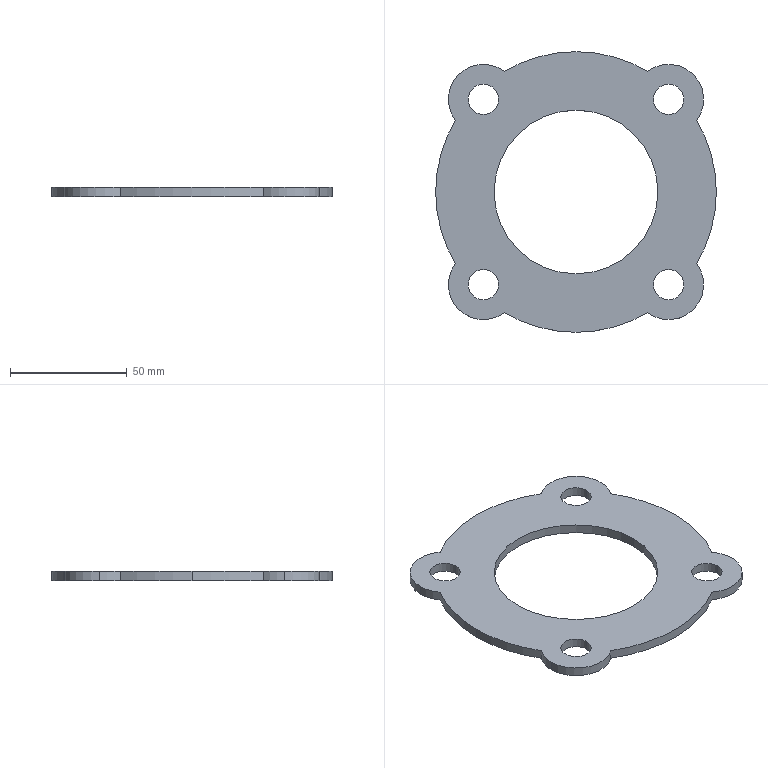Part | SolidWorks | features Extrusion 1 | 1 solid | 23 faces | box 120 x 120 x 4 mm | volume 31763 mm3 | cylinder 21 | plane 2 | commonest cylinder face diameters 13 x8 30 x6 120 x5 70 x2
STEP:
#1=CARTESIAN_POINT('',(-35.,0.,2.));
#2=VERTEX_POINT('',#1);
#3=CARTESIAN_POINT('',(35.,0.,2.));
#4=VERTEX_POINT('',#3);
#5=CARTESIAN_POINT('',(0.,0.,2.));
#6=DIRECTION('',(0.,0.,1.));
#7=DIRECTION('',(1.,0.,0.));
#8=AXIS2_PLACEMENT_3D('',#5,#6,#7);
#9=CIRCLE('',#8,35.);
#10=EDGE_CURVE('',#2,#4,#9,.T.);
#11=ORIENTED_EDGE('',*,*,#10,.T.);
#12=CARTESIAN_POINT('',(35.,0.,-2.));
#13=VERTEX_POINT('',#12);
#14=CARTESIAN_POINT('',(35.,0.,2.));
#15=DIRECTION('',(0.,0.,-1.));
#16=VECTOR('',#15,1000.);
#17=LINE('',#14,#16);
#18=EDGE_CURVE('',#4,#13,#17,.T.);
#19=ORIENTED_EDGE('',*,*,#18,.T.);
#20=CARTESIAN_POINT('',(-35.,0.,-2.));
#21=VERTEX_POINT('',#20);
#22=CARTESIAN_POINT('',(0.,0.,-2.));
#23=DIRECTION('',(0.,0.,1.));
#24=DIRECTION('',(1.,0.,0.));
#25=AXIS2_PLACEMENT_3D('',#22,#23,#24);
#26=CIRCLE('',#25,35.);
#27=EDGE_CURVE('',#21,#13,#26,.T.);
#28=ORIENTED_EDGE('',*,*,#27,.F.);
#29=CARTESIAN_POINT('',(-35.,0.,2.));
#30=DIRECTION('',(0.,0.,-1.));
#31=VECTOR('',#30,1000.);
#32=LINE('',#29,#31);
#33=EDGE_CURVE('',#2,#21,#32,.T.);
#34=ORIENTED_EDGE('',*,*,#33,.F.);
#35=EDGE_LOOP('',(#11,#19,#28,#34));
#36=FACE_OUTER_BOUND('',#35,.T.);
#37=CARTESIAN_POINT('',(0.,0.,2.));
#38=DIRECTION('',(0.,0.,-1.));
#39=DIRECTION('',(-1.,0.,0.));
#40=AXIS2_PLACEMENT_3D('',#37,#38,#39);
#41=CYLINDRICAL_SURFACE('',#40,35.);
#42=ADVANCED_FACE('',(#36),#41,.F.);
#43=CARTESIAN_POINT('',(33.098,39.598,2.));
#44=VERTEX_POINT('',#43);
#45=CARTESIAN_POINT('',(46.098,39.598,2.));
#46=VERTEX_POINT('',#45);
#47=CARTESIAN_POINT('',(39.598,39.598,2.));
#48=DIRECTION('',(0.,0.,1.));
#49=DIRECTION('',(1.,0.,0.));
#50=AXIS2_PLACEMENT_3D('',#47,#48,#49);
#51=CIRCLE('',#50,6.5);
#52=EDGE_CURVE('',#44,#46,#51,.T.);
#53=ORIENTED_EDGE('',*,*,#52,.T.);
#54=CARTESIAN_POINT('',(46.098,39.598,-2.));
#55=VERTEX_POINT('',#54);
#56=CARTESIAN_POINT('',(46.098,39.598,2.));
#57=DIRECTION('',(0.,0.,-1.));
#58=VECTOR('',#57,1000.);
#59=LINE('',#56,#58);
#60=EDGE_CURVE('',#46,#55,#59,.T.);
#61=ORIENTED_EDGE('',*,*,#60,.T.);
#62=CARTESIAN_POINT('',(33.098,39.598,-2.));
#63=VERTEX_POINT('',#62);
#64=CARTESIAN_POINT('',(39.598,39.598,-2.));
#65=DIRECTION('',(0.,0.,1.));
#66=DIRECTION('',(1.,0.,0.));
#67=AXIS2_PLACEMENT_3D('',#64,#65,#66);
#68=CIRCLE('',#67,6.5);
#69=EDGE_CURVE('',#63,#55,#68,.T.);
#70=ORIENTED_EDGE('',*,*,#69,.F.);
#71=CARTESIAN_POINT('',(33.098,39.598,2.));
#72=DIRECTION('',(0.,0.,-1.));
#73=VECTOR('',#72,1000.);
#74=LINE('',#71,#73);
#75=EDGE_CURVE('',#44,#63,#74,.T.);
#76=ORIENTED_EDGE('',*,*,#75,.F.);
#77=EDGE_LOOP('',(#53,#61,#70,#76));
#78=FACE_OUTER_BOUND('',#77,.T.);
#79=CARTESIAN_POINT('',(39.598,39.598,2.));
#80=DIRECTION('',(0.,0.,-1.));
#81=DIRECTION('',(-1.,0.,0.));
#82=AXIS2_PLACEMENT_3D('',#79,#80,#81);
#83=CYLINDRICAL_SURFACE('',#82,6.5);
#84=ADVANCED_FACE('',(#78),#83,.F.);
#85=CARTESIAN_POINT('',(33.098,-39.598,2.));
#86=VERTEX_POINT('',#85);
#87=CARTESIAN_POINT('',(46.098,-39.598,2.));
#88=VERTEX_POINT('',#87);
#89=CARTESIAN_POINT('',(39.598,-39.598,2.));
#90=DIRECTION('',(0.,0.,1.));
#91=DIRECTION('',(1.,0.,0.));
#92=AXIS2_PLACEMENT_3D('',#89,#90,#91);
#93=CIRCLE('',#92,6.5);
#94=EDGE_CURVE('',#86,#88,#93,.T.);
#95=ORIENTED_EDGE('',*,*,#94,.T.);
#96=CARTESIAN_POINT('',(46.098,-39.598,-2.));
#97=VERTEX_POINT('',#96);
#98=CARTESIAN_POINT('',(46.098,-39.598,2.));
#99=DIRECTION('',(0.,0.,-1.));
#100=VECTOR('',#99,1000.);
#101=LINE('',#98,#100);
#102=EDGE_CURVE('',#88,#97,#101,.T.);
#103=ORIENTED_EDGE('',*,*,#102,.T.);
#104=CARTESIAN_POINT('',(33.098,-39.598,-2.));
#105=VERTEX_POINT('',#104);
#106=CARTESIAN_POINT('',(39.598,-39.598,-2.));
#107=DIRECTION('',(0.,0.,1.));
#108=DIRECTION('',(1.,0.,0.));
#109=AXIS2_PLACEMENT_3D('',#106,#107,#108);
#110=CIRCLE('',#109,6.5);
#111=EDGE_CURVE('',#105,#97,#110,.T.);
#112=ORIENTED_EDGE('',*,*,#111,.F.);
#113=CARTESIAN_POINT('',(33.098,-39.598,2.));
#114=DIRECTION('',(0.,0.,-1.));
#115=VECTOR('',#114,1000.);
#116=LINE('',#113,#115);
#117=EDGE_CURVE('',#86,#105,#116,.T.);
#118=ORIENTED_EDGE('',*,*,#117,.F.);
#119=EDGE_LOOP('',(#95,#103,#112,#118));
#120=FACE_OUTER_BOUND('',#119,.T.);
#121=CARTESIAN_POINT('',(39.598,-39.598,2.));
#122=DIRECTION('',(0.,0.,-1.));
#123=DIRECTION('',(-1.,0.,0.));
#124=AXIS2_PLACEMENT_3D('',#121,#122,#123);
#125=CYLINDRICAL_SURFACE('',#124,6.5);
#126=ADVANCED_FACE('',(#120),#125,.F.);
#127=CARTESIAN_POINT('',(-46.098,-39.598,2.));
#128=VERTEX_POINT('',#127);
#129=CARTESIAN_POINT('',(-33.098,-39.598,2.));
#130=VERTEX_POINT('',#129);
#131=CARTESIAN_POINT('',(-39.598,-39.598,2.));
#132=DIRECTION('',(0.,0.,1.));
#133=DIRECTION('',(1.,0.,0.));
#134=AXIS2_PLACEMENT_3D('',#131,#132,#133);
#135=CIRCLE('',#134,6.5);
#136=EDGE_CURVE('',#128,#130,#135,.T.);
#137=ORIENTED_EDGE('',*,*,#136,.T.);
#138=CARTESIAN_POINT('',(-33.098,-39.598,-2.));
#139=VERTEX_POINT('',#138);
#140=CARTESIAN_POINT('',(-33.098,-39.598,2.));
#141=DIRECTION('',(0.,0.,-1.));
#142=VECTOR('',#141,1000.);
#143=LINE('',#140,#142);
#144=EDGE_CURVE('',#130,#139,#143,.T.);
#145=ORIENTED_EDGE('',*,*,#144,.T.);
#146=CARTESIAN_POINT('',(-46.098,-39.598,-2.));
#147=VERTEX_POINT('',#146);
#148=CARTESIAN_POINT('',(-39.598,-39.598,-2.));
#149=DIRECTION('',(0.,0.,1.));
#150=DIRECTION('',(1.,0.,0.));
#151=AXIS2_PLACEMENT_3D('',#148,#149,#150);
#152=CIRCLE('',#151,6.5);
#153=EDGE_CURVE('',#147,#139,#152,.T.);
#154=ORIENTED_EDGE('',*,*,#153,.F.);
#155=CARTESIAN_POINT('',(-46.098,-39.598,2.));
#156=DIRECTION('',(0.,0.,-1.));
#157=VECTOR('',#156,1000.);
#158=LINE('',#155,#157);
#159=EDGE_CURVE('',#128,#147,#158,.T.);
#160=ORIENTED_EDGE('',*,*,#159,.F.);
#161=EDGE_LOOP('',(#137,#145,#154,#160));
#162=FACE_OUTER_BOUND('',#161,.T.);
#163=CARTESIAN_POINT('',(-39.598,-39.598,2.));
#164=DIRECTION('',(0.,0.,-1.));
#165=DIRECTION('',(-1.,0.,0.));
#166=AXIS2_PLACEMENT_3D('',#163,#164,#165);
#167=CYLINDRICAL_SURFACE('',#166,6.5);
#168=ADVANCED_FACE('',(#162),#167,.F.);
#169=CARTESIAN_POINT('',(-46.098,39.598,2.));
#170=VERTEX_POINT('',#169);
#171=CARTESIAN_POINT('',(-33.098,39.598,2.));
#172=VERTEX_POINT('',#171);
#173=CARTESIAN_POINT('',(-39.598,39.598,2.));
#174=DIRECTION('',(0.,0.,1.));
#175=DIRECTION('',(1.,0.,0.));
#176=AXIS2_PLACEMENT_3D('',#173,#174,#175);
#177=CIRCLE('',#176,6.5);
#178=EDGE_CURVE('',#170,#172,#177,.T.);
#179=ORIENTED_EDGE('',*,*,#178,.T.);
#180=CARTESIAN_POINT('',(-33.098,39.598,-2.));
#181=VERTEX_POINT('',#180);
#182=CARTESIAN_POINT('',(-33.098,39.598,2.));
#183=DIRECTION('',(0.,0.,-1.));
#184=VECTOR('',#183,1000.);
#185=LINE('',#182,#184);
#186=EDGE_CURVE('',#172,#181,#185,.T.);
#187=ORIENTED_EDGE('',*,*,#186,.T.);
#188=CARTESIAN_POINT('',(-46.098,39.598,-2.));
#189=VERTEX_POINT('',#188);
#190=CARTESIAN_POINT('',(-39.598,39.598,-2.));
#191=DIRECTION('',(0.,0.,1.));
#192=DIRECTION('',(1.,0.,0.));
#193=AXIS2_PLACEMENT_3D('',#190,#191,#192);
#194=CIRCLE('',#193,6.5);
#195=EDGE_CURVE('',#189,#181,#194,.T.);
#196=ORIENTED_EDGE('',*,*,#195,.F.);
#197=CARTESIAN_POINT('',(-46.098,39.598,2.));
#198=DIRECTION('',(0.,0.,-1.));
#199=VECTOR('',#198,1000.);
#200=LINE('',#197,#199);
#201=EDGE_CURVE('',#170,#189,#200,.T.);
#202=ORIENTED_EDGE('',*,*,#201,.F.);
#203=EDGE_LOOP('',(#179,#187,#196,#202));
#204=FACE_OUTER_BOUND('',#203,.T.);
#205=CARTESIAN_POINT('',(-39.598,39.598,2.));
#206=DIRECTION('',(0.,0.,-1.));
#207=DIRECTION('',(-1.,0.,0.));
#208=AXIS2_PLACEMENT_3D('',#205,#206,#207);
#209=CYLINDRICAL_SURFACE('',#208,6.5);
#210=ADVANCED_FACE('',(#204),#209,.F.);
#211=CARTESIAN_POINT('',(-54.598,-39.598,2.));
#212=VERTEX_POINT('',#211);
#213=CARTESIAN_POINT('',(-30.608,-51.606,2.));
#214=VERTEX_POINT('',#213);
#215=CARTESIAN_POINT('',(-39.598,-39.598,2.));
#216=DIRECTION('',(0.,0.,1.));
#217=DIRECTION('',(1.,0.,0.));
#218=AXIS2_PLACEMENT_3D('',#215,#216,#217);
#219=CIRCLE('',#218,15.);
#220=EDGE_CURVE('',#212,#214,#219,.T.);
#221=ORIENTED_EDGE('',*,*,#220,.F.);
#222=CARTESIAN_POINT('',(-54.598,-39.598,-2.));
#223=VERTEX_POINT('',#222);
#224=CARTESIAN_POINT('',(-54.598,-39.598,2.));
#225=DIRECTION('',(0.,0.,-1.));
#226=VECTOR('',#225,1000.);
#227=LINE('',#224,#226);
#228=EDGE_CURVE('',#212,#223,#227,.T.);
#229=ORIENTED_EDGE('',*,*,#228,.T.);
#230=CARTESIAN_POINT('',(-30.608,-51.606,-2.));
#231=VERTEX_POINT('',#230);
#232=CARTESIAN_POINT('',(-39.598,-39.598,-2.));
#233=DIRECTION('',(0.,0.,1.));
#234=DIRECTION('',(1.,0.,0.));
#235=AXIS2_PLACEMENT_3D('',#232,#233,#234);
#236=CIRCLE('',#235,15.);
#237=EDGE_CURVE('',#223,#231,#236,.T.);
#238=ORIENTED_EDGE('',*,*,#237,.T.);
#239=CARTESIAN_POINT('',(-30.608,-51.606,2.));
#240=DIRECTION('',(0.,0.,-1.));
#241=VECTOR('',#240,1000.);
#242=LINE('',#239,#241);
#243=EDGE_CURVE('',#214,#231,#242,.T.);
#244=ORIENTED_EDGE('',*,*,#243,.F.);
#245=EDGE_LOOP('',(#221,#229,#238,#244));
#246=FACE_OUTER_BOUND('',#245,.T.);
#247=CARTESIAN_POINT('',(-39.598,-39.598,2.));
#248=DIRECTION('',(0.,0.,-1.));
#249=DIRECTION('',(-1.,0.,0.));
#250=AXIS2_PLACEMENT_3D('',#247,#248,#249);
#251=CYLINDRICAL_SURFACE('',#250,15.);
#252=ADVANCED_FACE('',(#246),#251,.T.);
#253=CARTESIAN_POINT('',(-60.,0.,2.));
#254=VERTEX_POINT('',#253);
#255=CARTESIAN_POINT('',(-51.606,-30.608,2.));
#256=VERTEX_POINT('',#255);
#257=CARTESIAN_POINT('',(0.,0.,2.));
#258=DIRECTION('',(0.,0.,1.));
#259=DIRECTION('',(1.,0.,0.));
#260=AXIS2_PLACEMENT_3D('',#257,#258,#259);
#261=CIRCLE('',#260,60.);
#262=EDGE_CURVE('',#254,#256,#261,.T.);
#263=ORIENTED_EDGE('',*,*,#262,.F.);
#264=CARTESIAN_POINT('',(-60.,0.,-2.));
#265=VERTEX_POINT('',#264);
#266=CARTESIAN_POINT('',(-60.,0.,2.));
#267=DIRECTION('',(0.,0.,-1.));
#268=VECTOR('',#267,1000.);
#269=LINE('',#266,#268);
#270=EDGE_CURVE('',#254,#265,#269,.T.);
#271=ORIENTED_EDGE('',*,*,#270,.T.);
#272=CARTESIAN_POINT('',(-51.606,-30.608,-2.));
#273=VERTEX_POINT('',#272);
#274=CARTESIAN_POINT('',(0.,0.,-2.));
#275=DIRECTION('',(0.,0.,1.));
#276=DIRECTION('',(1.,0.,0.));
#277=AXIS2_PLACEMENT_3D('',#274,#275,#276);
#278=CIRCLE('',#277,60.);
#279=EDGE_CURVE('',#265,#273,#278,.T.);
#280=ORIENTED_EDGE('',*,*,#279,.T.);
#281=CARTESIAN_POINT('',(-51.606,-30.608,2.));
#282=DIRECTION('',(0.,0.,-1.));
#283=VECTOR('',#282,1000.);
#284=LINE('',#281,#283);
#285=EDGE_CURVE('',#256,#273,#284,.T.);
#286=ORIENTED_EDGE('',*,*,#285,.F.);
#287=EDGE_LOOP('',(#263,#271,#280,#286));
#288=FACE_OUTER_BOUND('',#287,.T.);
#289=CARTESIAN_POINT('',(0.,0.,2.));
#290=DIRECTION('',(0.,0.,-1.));
#291=DIRECTION('',(-1.,0.,0.));
#292=AXIS2_PLACEMENT_3D('',#289,#290,#291);
#293=CYLINDRICAL_SURFACE('',#292,60.);
#294=ADVANCED_FACE('',(#288),#293,.T.);
#295=CARTESIAN_POINT('',(-54.598,39.598,2.));
#296=VERTEX_POINT('',#295);
#297=CARTESIAN_POINT('',(-51.606,30.608,2.));
#298=VERTEX_POINT('',#297);
#299=CARTESIAN_POINT('',(-39.598,39.598,2.));
#300=DIRECTION('',(0.,0.,1.));
#301=DIRECTION('',(1.,0.,0.));
#302=AXIS2_PLACEMENT_3D('',#299,#300,#301);
#303=CIRCLE('',#302,15.);
#304=EDGE_CURVE('',#296,#298,#303,.T.);
#305=ORIENTED_EDGE('',*,*,#304,.F.);
#306=CARTESIAN_POINT('',(-54.598,39.598,-2.));
#307=VERTEX_POINT('',#306);
#308=CARTESIAN_POINT('',(-54.598,39.598,2.));
#309=DIRECTION('',(0.,0.,-1.));
#310=VECTOR('',#309,1000.);
#311=LINE('',#308,#310);
#312=EDGE_CURVE('',#296,#307,#311,.T.);
#313=ORIENTED_EDGE('',*,*,#312,.T.);
#314=CARTESIAN_POINT('',(-51.606,30.608,-2.));
#315=VERTEX_POINT('',#314);
#316=CARTESIAN_POINT('',(-39.598,39.598,-2.));
#317=DIRECTION('',(0.,0.,1.));
#318=DIRECTION('',(1.,0.,0.));
#319=AXIS2_PLACEMENT_3D('',#316,#317,#318);
#320=CIRCLE('',#319,15.);
#321=EDGE_CURVE('',#307,#315,#320,.T.);
#322=ORIENTED_EDGE('',*,*,#321,.T.);
#323=CARTESIAN_POINT('',(-51.606,30.608,2.));
#324=DIRECTION('',(0.,0.,-1.));
#325=VECTOR('',#324,1000.);
#326=LINE('',#323,#325);
#327=EDGE_CURVE('',#298,#315,#326,.T.);
#328=ORIENTED_EDGE('',*,*,#327,.F.);
#329=EDGE_LOOP('',(#305,#313,#322,#328));
#330=FACE_OUTER_BOUND('',#329,.T.);
#331=CARTESIAN_POINT('',(-39.598,39.598,2.));
#332=DIRECTION('',(0.,0.,-1.));
#333=DIRECTION('',(-1.,0.,0.));
#334=AXIS2_PLACEMENT_3D('',#331,#332,#333);
#335=CYLINDRICAL_SURFACE('',#334,15.);
#336=ADVANCED_FACE('',(#330),#335,.T.);
#337=CARTESIAN_POINT('',(30.608,-51.606,-2.));
#338=VERTEX_POINT('',#337);
#339=CARTESIAN_POINT('',(51.606,-30.608,-2.));
#340=VERTEX_POINT('',#339);
#341=CARTESIAN_POINT('',(39.598,-39.598,-2.));
#342=DIRECTION('',(0.,0.,1.));
#343=DIRECTION('',(1.,0.,0.));
#344=AXIS2_PLACEMENT_3D('',#341,#342,#343);
#345=CIRCLE('',#344,15.);
#346=EDGE_CURVE('',#338,#340,#345,.T.);
#347=ORIENTED_EDGE('',*,*,#346,.T.);
#348=CARTESIAN_POINT('',(51.606,-30.608,2.));
#349=VERTEX_POINT('',#348);
#350=CARTESIAN_POINT('',(51.606,-30.608,2.));
#351=DIRECTION('',(0.,0.,-1.));
#352=VECTOR('',#351,1000.);
#353=LINE('',#350,#352);
#354=EDGE_CURVE('',#349,#340,#353,.T.);
#355=ORIENTED_EDGE('',*,*,#354,.F.);
#356=CARTESIAN_POINT('',(30.608,-51.606,2.));
#357=VERTEX_POINT('',#356);
#358=CARTESIAN_POINT('',(39.598,-39.598,2.));
#359=DIRECTION('',(0.,0.,1.));
#360=DIRECTION('',(1.,0.,0.));
#361=AXIS2_PLACEMENT_3D('',#358,#359,#360);
#362=CIRCLE('',#361,15.);
#363=EDGE_CURVE('',#357,#349,#362,.T.);
#364=ORIENTED_EDGE('',*,*,#363,.F.);
#365=CARTESIAN_POINT('',(30.608,-51.606,2.));
#366=DIRECTION('',(0.,0.,-1.));
#367=VECTOR('',#366,1000.);
#368=LINE('',#365,#367);
#369=EDGE_CURVE('',#357,#338,#368,.T.);
#370=ORIENTED_EDGE('',*,*,#369,.T.);
#371=EDGE_LOOP('',(#347,#355,#364,#370));
#372=FACE_OUTER_BOUND('',#371,.T.);
#373=CARTESIAN_POINT('',(39.598,-39.598,2.));
#374=DIRECTION('',(0.,0.,-1.));
#375=DIRECTION('',(-1.,0.,0.));
#376=AXIS2_PLACEMENT_3D('',#373,#374,#375);
#377=CYLINDRICAL_SURFACE('',#376,15.);
#378=ADVANCED_FACE('',(#372),#377,.T.);
#379=CARTESIAN_POINT('',(51.606,30.608,-2.));
#380=VERTEX_POINT('',#379);
#381=CARTESIAN_POINT('',(0.,0.,-2.));
#382=DIRECTION('',(0.,0.,1.));
#383=DIRECTION('',(1.,0.,0.));
#384=AXIS2_PLACEMENT_3D('',#381,#382,#383);
#385=CIRCLE('',#384,60.);
#386=EDGE_CURVE('',#340,#380,#385,.T.);
#387=ORIENTED_EDGE('',*,*,#386,.T.);
#388=CARTESIAN_POINT('',(51.606,30.608,2.));
#389=VERTEX_POINT('',#388);
#390=CARTESIAN_POINT('',(51.606,30.608,2.));
#391=DIRECTION('',(0.,0.,-1.));
#392=VECTOR('',#391,1000.);
#393=LINE('',#390,#392);
#394=EDGE_CURVE('',#389,#380,#393,.T.);
#395=ORIENTED_EDGE('',*,*,#394,.F.);
#396=CARTESIAN_POINT('',(0.,0.,2.));
#397=DIRECTION('',(0.,0.,1.));
#398=DIRECTION('',(1.,0.,0.));
#399=AXIS2_PLACEMENT_3D('',#396,#397,#398);
#400=CIRCLE('',#399,60.);
#401=EDGE_CURVE('',#349,#389,#400,.T.);
#402=ORIENTED_EDGE('',*,*,#401,.F.);
#403=ORIENTED_EDGE('',*,*,#354,.T.);
#404=EDGE_LOOP('',(#387,#395,#402,#403));
#405=FACE_OUTER_BOUND('',#404,.T.);
#406=CARTESIAN_POINT('',(0.,0.,2.));
#407=DIRECTION('',(0.,0.,-1.));
#408=DIRECTION('',(-1.,0.,0.));
#409=AXIS2_PLACEMENT_3D('',#406,#407,#408);
#410=CYLINDRICAL_SURFACE('',#409,60.);
#411=ADVANCED_FACE('',(#405),#410,.T.);
#412=CARTESIAN_POINT('',(30.608,51.606,-2.));
#413=VERTEX_POINT('',#412);
#414=CARTESIAN_POINT('',(39.598,39.598,-2.));
#415=DIRECTION('',(0.,0.,1.));
#416=DIRECTION('',(1.,0.,0.));
#417=AXIS2_PLACEMENT_3D('',#414,#415,#416);
#418=CIRCLE('',#417,15.);
#419=EDGE_CURVE('',#380,#413,#418,.T.);
#420=ORIENTED_EDGE('',*,*,#419,.T.);
#421=CARTESIAN_POINT('',(30.608,51.606,2.));
#422=VERTEX_POINT('',#421);
#423=CARTESIAN_POINT('',(30.608,51.606,2.));
#424=DIRECTION('',(0.,0.,-1.));
#425=VECTOR('',#424,1000.);
#426=LINE('',#423,#425);
#427=EDGE_CURVE('',#422,#413,#426,.T.);
#428=ORIENTED_EDGE('',*,*,#427,.F.);
#429=CARTESIAN_POINT('',(39.598,39.598,2.));
#430=DIRECTION('',(0.,0.,1.));
#431=DIRECTION('',(1.,0.,0.));
#432=AXIS2_PLACEMENT_3D('',#429,#430,#431);
#433=CIRCLE('',#432,15.);
#434=EDGE_CURVE('',#389,#422,#433,.T.);
#435=ORIENTED_EDGE('',*,*,#434,.F.);
#436=ORIENTED_EDGE('',*,*,#394,.T.);
#437=EDGE_LOOP('',(#420,#428,#435,#436));
#438=FACE_OUTER_BOUND('',#437,.T.);
#439=CARTESIAN_POINT('',(39.598,39.598,2.));
#440=DIRECTION('',(0.,0.,-1.));
#441=DIRECTION('',(-1.,0.,0.));
#442=AXIS2_PLACEMENT_3D('',#439,#440,#441);
#443=CYLINDRICAL_SURFACE('',#442,15.);
#444=ADVANCED_FACE('',(#438),#443,.T.);
#445=CARTESIAN_POINT('',(-30.608,51.606,-2.));
#446=VERTEX_POINT('',#445);
#447=CARTESIAN_POINT('',(0.,0.,-2.));
#448=DIRECTION('',(0.,0.,1.));
#449=DIRECTION('',(1.,0.,0.));
#450=AXIS2_PLACEMENT_3D('',#447,#448,#449);
#451=CIRCLE('',#450,60.);
#452=EDGE_CURVE('',#413,#446,#451,.T.);
#453=ORIENTED_EDGE('',*,*,#452,.T.);
#454=CARTESIAN_POINT('',(-30.608,51.606,2.));
#455=VERTEX_POINT('',#454);
#456=CARTESIAN_POINT('',(-30.608,51.606,2.));
#457=DIRECTION('',(0.,0.,-1.));
#458=VECTOR('',#457,1000.);
#459=LINE('',#456,#458);
#460=EDGE_CURVE('',#455,#446,#459,.T.);
#461=ORIENTED_EDGE('',*,*,#460,.F.);
#462=CARTESIAN_POINT('',(0.,0.,2.));
#463=DIRECTION('',(0.,0.,1.));
#464=DIRECTION('',(1.,0.,0.));
#465=AXIS2_PLACEMENT_3D('',#462,#463,#464);
#466=CIRCLE('',#465,60.);
#467=EDGE_CURVE('',#422,#455,#466,.T.);
#468=ORIENTED_EDGE('',*,*,#467,.F.);
#469=ORIENTED_EDGE('',*,*,#427,.T.);
#470=EDGE_LOOP('',(#453,#461,#468,#469));
#471=FACE_OUTER_BOUND('',#470,.T.);
#472=CARTESIAN_POINT('',(0.,0.,2.));
#473=DIRECTION('',(0.,0.,-1.));
#474=DIRECTION('',(-1.,0.,0.));
#475=AXIS2_PLACEMENT_3D('',#472,#473,#474);
#476=CYLINDRICAL_SURFACE('',#475,60.);
#477=ADVANCED_FACE('',(#471),#476,.T.);
#478=ORIENTED_EDGE('',*,*,#312,.F.);
#479=CARTESIAN_POINT('',(-39.598,39.598,2.));
#480=DIRECTION('',(0.,0.,1.));
#481=DIRECTION('',(1.,0.,0.));
#482=AXIS2_PLACEMENT_3D('',#479,#480,#481);
#483=CIRCLE('',#482,15.);
#484=EDGE_CURVE('',#455,#296,#483,.T.);
#485=ORIENTED_EDGE('',*,*,#484,.F.);
#486=ORIENTED_EDGE('',*,*,#460,.T.);
#487=CARTESIAN_POINT('',(-39.598,39.598,-2.));
#488=DIRECTION('',(0.,0.,1.));
#489=DIRECTION('',(1.,0.,0.));
#490=AXIS2_PLACEMENT_3D('',#487,#488,#489);
#491=CIRCLE('',#490,15.);
#492=EDGE_CURVE('',#446,#307,#491,.T.);
#493=ORIENTED_EDGE('',*,*,#492,.T.);
#494=EDGE_LOOP('',(#478,#485,#486,#493));
#495=FACE_OUTER_BOUND('',#494,.T.);
#496=CARTESIAN_POINT('',(-39.598,39.598,2.));
#497=DIRECTION('',(0.,0.,-1.));
#498=DIRECTION('',(-1.,0.,0.));
#499=AXIS2_PLACEMENT_3D('',#496,#497,#498);
#500=CYLINDRICAL_SURFACE('',#499,15.);
#501=ADVANCED_FACE('',(#495),#500,.T.);
#502=ORIENTED_EDGE('',*,*,#270,.F.);
#503=CARTESIAN_POINT('',(0.,0.,2.));
#504=DIRECTION('',(0.,0.,1.));
#505=DIRECTION('',(1.,0.,0.));
#506=AXIS2_PLACEMENT_3D('',#503,#504,#505);
#507=CIRCLE('',#506,60.);
#508=EDGE_CURVE('',#298,#254,#507,.T.);
#509=ORIENTED_EDGE('',*,*,#508,.F.);
#510=ORIENTED_EDGE('',*,*,#327,.T.);
#511=CARTESIAN_POINT('',(0.,0.,-2.));
#512=DIRECTION('',(0.,0.,1.));
#513=DIRECTION('',(1.,0.,0.));
#514=AXIS2_PLACEMENT_3D('',#511,#512,#513);
#515=CIRCLE('',#514,60.);
#516=EDGE_CURVE('',#315,#265,#515,.T.);
#517=ORIENTED_EDGE('',*,*,#516,.T.);
#518=EDGE_LOOP('',(#502,#509,#510,#517));
#519=FACE_OUTER_BOUND('',#518,.T.);
#520=CARTESIAN_POINT('',(0.,0.,2.));
#521=DIRECTION('',(0.,0.,-1.));
#522=DIRECTION('',(-1.,0.,0.));
#523=AXIS2_PLACEMENT_3D('',#520,#521,#522);
#524=CYLINDRICAL_SURFACE('',#523,60.);
#525=ADVANCED_FACE('',(#519),#524,.T.);
#526=ORIENTED_EDGE('',*,*,#228,.F.);
#527=CARTESIAN_POINT('',(-39.598,-39.598,2.));
#528=DIRECTION('',(0.,0.,1.));
#529=DIRECTION('',(1.,0.,0.));
#530=AXIS2_PLACEMENT_3D('',#527,#528,#529);
#531=CIRCLE('',#530,15.);
#532=EDGE_CURVE('',#256,#212,#531,.T.);
#533=ORIENTED_EDGE('',*,*,#532,.F.);
#534=ORIENTED_EDGE('',*,*,#285,.T.);
#535=CARTESIAN_POINT('',(-39.598,-39.598,-2.));
#536=DIRECTION('',(0.,0.,1.));
#537=DIRECTION('',(1.,0.,0.));
#538=AXIS2_PLACEMENT_3D('',#535,#536,#537);
#539=CIRCLE('',#538,15.);
#540=EDGE_CURVE('',#273,#223,#539,.T.);
#541=ORIENTED_EDGE('',*,*,#540,.T.);
#542=EDGE_LOOP('',(#526,#533,#534,#541));
#543=FACE_OUTER_BOUND('',#542,.T.);
#544=CARTESIAN_POINT('',(-39.598,-39.598,2.));
#545=DIRECTION('',(0.,0.,-1.));
#546=DIRECTION('',(-1.,0.,0.));
#547=AXIS2_PLACEMENT_3D('',#544,#545,#546);
#548=CYLINDRICAL_SURFACE('',#547,15.);
#549=ADVANCED_FACE('',(#543),#548,.T.);
#550=ORIENTED_EDGE('',*,*,#186,.F.);
#551=CARTESIAN_POINT('',(-39.598,39.598,2.));
#552=DIRECTION('',(0.,0.,1.));
#553=DIRECTION('',(1.,0.,0.));
#554=AXIS2_PLACEMENT_3D('',#551,#552,#553);
#555=CIRCLE('',#554,6.5);
#556=EDGE_CURVE('',#172,#170,#555,.T.);
#557=ORIENTED_EDGE('',*,*,#556,.T.);
#558=ORIENTED_EDGE('',*,*,#201,.T.);
#559=CARTESIAN_POINT('',(-39.598,39.598,-2.));
#560=DIRECTION('',(0.,0.,1.));
#561=DIRECTION('',(1.,0.,0.));
#562=AXIS2_PLACEMENT_3D('',#559,#560,#561);
#563=CIRCLE('',#562,6.5);
#564=EDGE_CURVE('',#181,#189,#563,.T.);
#565=ORIENTED_EDGE('',*,*,#564,.F.);
#566=EDGE_LOOP('',(#550,#557,#558,#565));
#567=FACE_OUTER_BOUND('',#566,.T.);
#568=CARTESIAN_POINT('',(-39.598,39.598,2.));
#569=DIRECTION('',(0.,0.,-1.));
#570=DIRECTION('',(-1.,0.,0.));
#571=AXIS2_PLACEMENT_3D('',#568,#569,#570);
#572=CYLINDRICAL_SURFACE('',#571,6.5);
#573=ADVANCED_FACE('',(#567),#572,.F.);
#574=ORIENTED_EDGE('',*,*,#144,.F.);
#575=CARTESIAN_POINT('',(-39.598,-39.598,2.));
#576=DIRECTION('',(0.,0.,1.));
#577=DIRECTION('',(1.,0.,0.));
#578=AXIS2_PLACEMENT_3D('',#575,#576,#577);
#579=CIRCLE('',#578,6.5);
#580=EDGE_CURVE('',#130,#128,#579,.T.);
#581=ORIENTED_EDGE('',*,*,#580,.T.);
#582=ORIENTED_EDGE('',*,*,#159,.T.);
#583=CARTESIAN_POINT('',(-39.598,-39.598,-2.));
#584=DIRECTION('',(0.,0.,1.));
#585=DIRECTION('',(1.,0.,0.));
#586=AXIS2_PLACEMENT_3D('',#583,#584,#585);
#587=CIRCLE('',#586,6.5);
#588=EDGE_CURVE('',#139,#147,#587,.T.);
#589=ORIENTED_EDGE('',*,*,#588,.F.);
#590=EDGE_LOOP('',(#574,#581,#582,#589));
#591=FACE_OUTER_BOUND('',#590,.T.);
#592=CARTESIAN_POINT('',(-39.598,-39.598,2.));
#593=DIRECTION('',(0.,0.,-1.));
#594=DIRECTION('',(-1.,0.,0.));
#595=AXIS2_PLACEMENT_3D('',#592,#593,#594);
#596=CYLINDRICAL_SURFACE('',#595,6.5);
#597=ADVANCED_FACE('',(#591),#596,.F.);
#598=ORIENTED_EDGE('',*,*,#102,.F.);
#599=CARTESIAN_POINT('',(39.598,-39.598,2.));
#600=DIRECTION('',(0.,0.,1.));
#601=DIRECTION('',(1.,0.,0.));
#602=AXIS2_PLACEMENT_3D('',#599,#600,#601);
#603=CIRCLE('',#602,6.5);
#604=EDGE_CURVE('',#88,#86,#603,.T.);
#605=ORIENTED_EDGE('',*,*,#604,.T.);
#606=ORIENTED_EDGE('',*,*,#117,.T.);
#607=CARTESIAN_POINT('',(39.598,-39.598,-2.));
#608=DIRECTION('',(0.,0.,1.));
#609=DIRECTION('',(1.,0.,0.));
#610=AXIS2_PLACEMENT_3D('',#607,#608,#609);
#611=CIRCLE('',#610,6.5);
#612=EDGE_CURVE('',#97,#105,#611,.T.);
#613=ORIENTED_EDGE('',*,*,#612,.F.);
#614=EDGE_LOOP('',(#598,#605,#606,#613));
#615=FACE_OUTER_BOUND('',#614,.T.);
#616=CARTESIAN_POINT('',(39.598,-39.598,2.));
#617=DIRECTION('',(0.,0.,-1.));
#618=DIRECTION('',(-1.,0.,0.));
#619=AXIS2_PLACEMENT_3D('',#616,#617,#618);
#620=CYLINDRICAL_SURFACE('',#619,6.5);
#621=ADVANCED_FACE('',(#615),#620,.F.);
#622=ORIENTED_EDGE('',*,*,#60,.F.);
#623=CARTESIAN_POINT('',(39.598,39.598,2.));
#624=DIRECTION('',(0.,0.,1.));
#625=DIRECTION('',(1.,0.,0.));
#626=AXIS2_PLACEMENT_3D('',#623,#624,#625);
#627=CIRCLE('',#626,6.5);
#628=EDGE_CURVE('',#46,#44,#627,.T.);
#629=ORIENTED_EDGE('',*,*,#628,.T.);
#630=ORIENTED_EDGE('',*,*,#75,.T.);
#631=CARTESIAN_POINT('',(39.598,39.598,-2.));
#632=DIRECTION('',(0.,0.,1.));
#633=DIRECTION('',(1.,0.,0.));
#634=AXIS2_PLACEMENT_3D('',#631,#632,#633);
#635=CIRCLE('',#634,6.5);
#636=EDGE_CURVE('',#55,#63,#635,.T.);
#637=ORIENTED_EDGE('',*,*,#636,.F.);
#638=EDGE_LOOP('',(#622,#629,#630,#637));
#639=FACE_OUTER_BOUND('',#638,.T.);
#640=CARTESIAN_POINT('',(39.598,39.598,2.));
#641=DIRECTION('',(0.,0.,-1.));
#642=DIRECTION('',(-1.,0.,0.));
#643=AXIS2_PLACEMENT_3D('',#640,#641,#642);
#644=CYLINDRICAL_SURFACE('',#643,6.5);
#645=ADVANCED_FACE('',(#639),#644,.F.);
#646=ORIENTED_EDGE('',*,*,#18,.F.);
#647=CARTESIAN_POINT('',(0.,0.,2.));
#648=DIRECTION('',(0.,0.,1.));
#649=DIRECTION('',(1.,0.,0.));
#650=AXIS2_PLACEMENT_3D('',#647,#648,#649);
#651=CIRCLE('',#650,35.);
#652=EDGE_CURVE('',#4,#2,#651,.T.);
#653=ORIENTED_EDGE('',*,*,#652,.T.);
#654=ORIENTED_EDGE('',*,*,#33,.T.);
#655=CARTESIAN_POINT('',(0.,0.,-2.));
#656=DIRECTION('',(0.,0.,1.));
#657=DIRECTION('',(1.,0.,0.));
#658=AXIS2_PLACEMENT_3D('',#655,#656,#657);
#659=CIRCLE('',#658,35.);
#660=EDGE_CURVE('',#13,#21,#659,.T.);
#661=ORIENTED_EDGE('',*,*,#660,.F.);
#662=EDGE_LOOP('',(#646,#653,#654,#661));
#663=FACE_OUTER_BOUND('',#662,.T.);
#664=CARTESIAN_POINT('',(0.,0.,2.));
#665=DIRECTION('',(0.,0.,-1.));
#666=DIRECTION('',(-1.,0.,0.));
#667=AXIS2_PLACEMENT_3D('',#664,#665,#666);
#668=CYLINDRICAL_SURFACE('',#667,35.);
#669=ADVANCED_FACE('',(#663),#668,.F.);
#670=CARTESIAN_POINT('',(0.,0.,-2.));
#671=DIRECTION('',(0.,0.,1.));
#672=DIRECTION('',(1.,0.,0.));
#673=AXIS2_PLACEMENT_3D('',#670,#671,#672);
#674=CIRCLE('',#673,60.);
#675=EDGE_CURVE('',#231,#338,#674,.T.);
#676=ORIENTED_EDGE('',*,*,#675,.T.);
#677=ORIENTED_EDGE('',*,*,#369,.F.);
#678=CARTESIAN_POINT('',(0.,0.,2.));
#679=DIRECTION('',(0.,0.,1.));
#680=DIRECTION('',(1.,0.,0.));
#681=AXIS2_PLACEMENT_3D('',#678,#679,#680);
#682=CIRCLE('',#681,60.);
#683=EDGE_CURVE('',#214,#357,#682,.T.);
#684=ORIENTED_EDGE('',*,*,#683,.F.);
#685=ORIENTED_EDGE('',*,*,#243,.T.);
#686=EDGE_LOOP('',(#676,#677,#684,#685));
#687=FACE_OUTER_BOUND('',#686,.T.);
#688=CARTESIAN_POINT('',(0.,0.,2.));
#689=DIRECTION('',(0.,0.,-1.));
#690=DIRECTION('',(-1.,0.,0.));
#691=AXIS2_PLACEMENT_3D('',#688,#689,#690);
#692=CYLINDRICAL_SURFACE('',#691,60.);
#693=ADVANCED_FACE('',(#687),#692,.T.);
#694=ORIENTED_EDGE('',*,*,#10,.F.);
#695=ORIENTED_EDGE('',*,*,#652,.F.);
#696=EDGE_LOOP('',(#694,#695));
#697=FACE_BOUND('',#696,.T.);
#698=ORIENTED_EDGE('',*,*,#52,.F.);
#699=ORIENTED_EDGE('',*,*,#628,.F.);
#700=EDGE_LOOP('',(#698,#699));
#701=FACE_BOUND('',#700,.T.);
#702=ORIENTED_EDGE('',*,*,#94,.F.);
#703=ORIENTED_EDGE('',*,*,#604,.F.);
#704=EDGE_LOOP('',(#702,#703));
#705=FACE_BOUND('',#704,.T.);
#706=ORIENTED_EDGE('',*,*,#136,.F.);
#707=ORIENTED_EDGE('',*,*,#580,.F.);
#708=EDGE_LOOP('',(#706,#707));
#709=FACE_BOUND('',#708,.T.);
#710=ORIENTED_EDGE('',*,*,#178,.F.);
#711=ORIENTED_EDGE('',*,*,#556,.F.);
#712=EDGE_LOOP('',(#710,#711));
#713=FACE_BOUND('',#712,.T.);
#714=ORIENTED_EDGE('',*,*,#363,.T.);
#715=ORIENTED_EDGE('',*,*,#401,.T.);
#716=ORIENTED_EDGE('',*,*,#434,.T.);
#717=ORIENTED_EDGE('',*,*,#467,.T.);
#718=ORIENTED_EDGE('',*,*,#484,.T.);
#719=ORIENTED_EDGE('',*,*,#304,.T.);
#720=ORIENTED_EDGE('',*,*,#508,.T.);
#721=ORIENTED_EDGE('',*,*,#262,.T.);
#722=ORIENTED_EDGE('',*,*,#532,.T.);
#723=ORIENTED_EDGE('',*,*,#220,.T.);
#724=ORIENTED_EDGE('',*,*,#683,.T.);
#725=EDGE_LOOP('',(#714,#715,#716,#717,#718,#719,#720,#721,#722,#723,#724));
#726=FACE_OUTER_BOUND('',#725,.T.);
#727=CARTESIAN_POINT('',(0.,0.,2.));
#728=DIRECTION('',(0.,0.,1.));
#729=DIRECTION('',(1.,0.,0.));
#730=AXIS2_PLACEMENT_3D('',#727,#728,#729);
#731=PLANE('',#730);
#732=ADVANCED_FACE('',(#697,#701,#705,#709,#713,#726),#731,.T.);
#733=ORIENTED_EDGE('',*,*,#27,.T.);
#734=ORIENTED_EDGE('',*,*,#660,.T.);
#735=EDGE_LOOP('',(#733,#734));
#736=FACE_BOUND('',#735,.T.);
#737=ORIENTED_EDGE('',*,*,#69,.T.);
#738=ORIENTED_EDGE('',*,*,#636,.T.);
#739=EDGE_LOOP('',(#737,#738));
#740=FACE_BOUND('',#739,.T.);
#741=ORIENTED_EDGE('',*,*,#111,.T.);
#742=ORIENTED_EDGE('',*,*,#612,.T.);
#743=EDGE_LOOP('',(#741,#742));
#744=FACE_BOUND('',#743,.T.);
#745=ORIENTED_EDGE('',*,*,#153,.T.);
#746=ORIENTED_EDGE('',*,*,#588,.T.);
#747=EDGE_LOOP('',(#745,#746));
#748=FACE_BOUND('',#747,.T.);
#749=ORIENTED_EDGE('',*,*,#195,.T.);
#750=ORIENTED_EDGE('',*,*,#564,.T.);
#751=EDGE_LOOP('',(#749,#750));
#752=FACE_BOUND('',#751,.T.);
#753=ORIENTED_EDGE('',*,*,#346,.F.);
#754=ORIENTED_EDGE('',*,*,#675,.F.);
#755=ORIENTED_EDGE('',*,*,#237,.F.);
#756=ORIENTED_EDGE('',*,*,#540,.F.);
#757=ORIENTED_EDGE('',*,*,#279,.F.);
#758=ORIENTED_EDGE('',*,*,#516,.F.);
#759=ORIENTED_EDGE('',*,*,#321,.F.);
#760=ORIENTED_EDGE('',*,*,#492,.F.);
#761=ORIENTED_EDGE('',*,*,#452,.F.);
#762=ORIENTED_EDGE('',*,*,#419,.F.);
#763=ORIENTED_EDGE('',*,*,#386,.F.);
#764=EDGE_LOOP('',(#753,#754,#755,#756,#757,#758,#759,#760,#761,#762,#763));
#765=FACE_OUTER_BOUND('',#764,.T.);
#766=CARTESIAN_POINT('',(0.,0.,-2.));
#767=DIRECTION('',(0.,0.,1.));
#768=DIRECTION('',(1.,0.,0.));
#769=AXIS2_PLACEMENT_3D('',#766,#767,#768);
#770=PLANE('',#769);
#771=ADVANCED_FACE('',(#736,#740,#744,#748,#752,#765),#770,.F.);
#772=CLOSED_SHELL('',(#42,#84,#126,#168,#210,#252,#294,#336,#378,#411,#444,#477,#501,#525,#549,#573,#597,#621,#645,#669,#693,#732,#771));
#773=MANIFOLD_SOLID_BREP('',#772);
#774=CARTESIAN_POINT('',(0.,0.,0.));
#775=DIRECTION('',(0.,0.,1.));
#776=DIRECTION('',(1.,0.,0.));
#777=AXIS2_PLACEMENT_3D('',#774,#775,#776);
#778=(LENGTH_UNIT()NAMED_UNIT(*)SI_UNIT(.MILLI.,.METRE.));
#779=UNCERTAINTY_MEASURE_WITH_UNIT(LENGTH_MEASURE(0.00001),#778,'','');
#780=(NAMED_UNIT(*)PLANE_ANGLE_UNIT()SI_UNIT($,.RADIAN.));
#781=(NAMED_UNIT(*)SI_UNIT($,.STERADIAN.)SOLID_ANGLE_UNIT());
#782=(GEOMETRIC_REPRESENTATION_CONTEXT(3)GLOBAL_UNCERTAINTY_ASSIGNED_CONTEXT((#779))GLOBAL_UNIT_ASSIGNED_CONTEXT((#778,#780,#781))REPRESENTATION_CONTEXT('',''));
#783=ADVANCED_BREP_SHAPE_REPRESENTATION('',(#773,#777),#782);